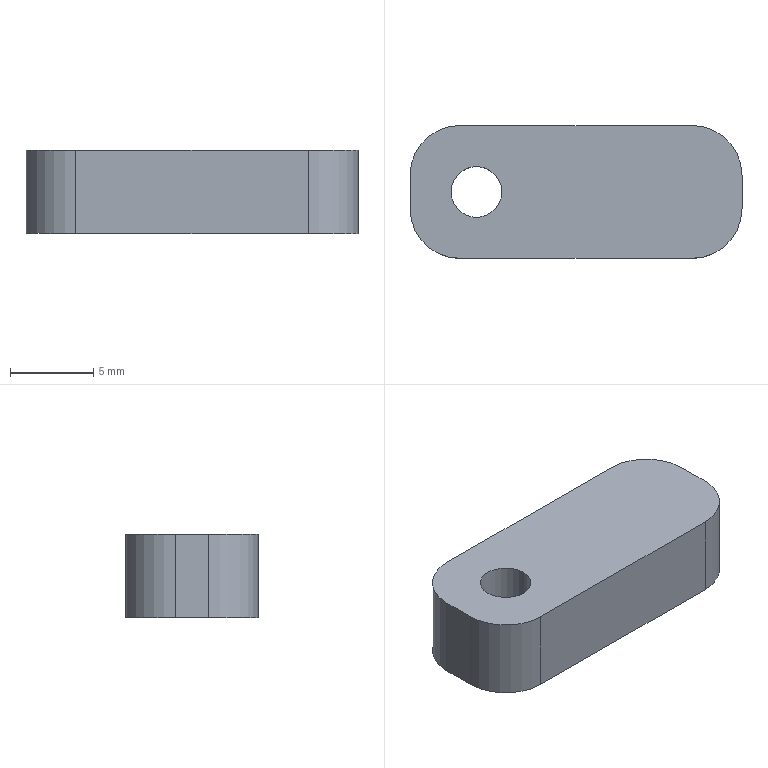Part | STEP file | ASND-0110-7.2aq | 1 solid | 12 faces | box 20 x 8 x 5 mm | volume 724.735 mm3 | cylinder 6 | plane 6 | commonest cylinder face diameters 6 x4 3.054 x2
STEP:
#1=CARTESIAN_POINT('',(0.,0.,0.));
#2=DIRECTION('',(0.,0.,1.));
#3=DIRECTION('',(1.,0.,0.));
#4=AXIS2_PLACEMENT_3D('',#1,#2,#3);
#5=CARTESIAN_POINT('',(-7.527,0.,5.));
#6=VERTEX_POINT('',#5);
#7=CARTESIAN_POINT('',(-7.527,0.,0.));
#8=VERTEX_POINT('',#7);
#9=CARTESIAN_POINT('',(-7.527,0.,5.));
#10=DIRECTION('',(0.,0.,-1.));
#11=VECTOR('',#10,1.);
#12=LINE('',#9,#11);
#13=CARTESIAN_POINT('',(-6.,0.,5.));
#14=DIRECTION('',(0.,0.,-1.));
#15=DIRECTION('',(-1.,0.,0.));
#16=AXIS2_PLACEMENT_3D('',#13,#14,#15);
#17=CYLINDRICAL_SURFACE('',#16,1.527);
#18=CARTESIAN_POINT('',(6.283,0.));
#19=DIRECTION('',(0.,1.));
#20=VECTOR('',#19,1.);
#21=LINE('',#18,#20);
#22=(GEOMETRIC_REPRESENTATION_CONTEXT(2)PARAMETRIC_REPRESENTATION_CONTEXT()REPRESENTATION_CONTEXT('',''));
#23=DEFINITIONAL_REPRESENTATION('',(#21),#22);
#24=PCURVE('',#17,#23);
#25=CARTESIAN_POINT('',(-6.,0.,5.));
#26=DIRECTION('',(0.,0.,-1.));
#27=DIRECTION('',(-1.,0.,0.));
#28=AXIS2_PLACEMENT_3D('',#25,#26,#27);
#29=CYLINDRICAL_SURFACE('',#28,1.527);
#30=CARTESIAN_POINT('',(0.,0.));
#31=DIRECTION('',(0.,1.));
#32=VECTOR('',#31,1.);
#33=LINE('',#30,#32);
#34=(GEOMETRIC_REPRESENTATION_CONTEXT(2)PARAMETRIC_REPRESENTATION_CONTEXT()REPRESENTATION_CONTEXT('',''));
#35=DEFINITIONAL_REPRESENTATION('',(#33),#34);
#36=PCURVE('',#29,#35);
#37=SURFACE_CURVE('',#12,(#24,#36),.PCURVE_S1.);
#38=EDGE_CURVE('',#6,#8,#37,.T.);
#39=ORIENTED_EDGE('',*,*,#38,.T.);
#40=CARTESIAN_POINT('',(-4.473,0.,0.));
#41=VERTEX_POINT('',#40);
#42=CARTESIAN_POINT('',(-6.,0.,0.));
#43=DIRECTION('',(0.,0.,1.));
#44=DIRECTION('',(1.,0.,0.));
#45=AXIS2_PLACEMENT_3D('',#42,#43,#44);
#46=CIRCLE('',#45,1.527);
#47=CARTESIAN_POINT('',(9.425,5.));
#48=DIRECTION('',(-1.,0.));
#49=VECTOR('',#48,1.);
#50=LINE('',#47,#49);
#51=(GEOMETRIC_REPRESENTATION_CONTEXT(2)PARAMETRIC_REPRESENTATION_CONTEXT()REPRESENTATION_CONTEXT('',''));
#52=DEFINITIONAL_REPRESENTATION('',(#50),#51);
#53=PCURVE('',#17,#52);
#54=CARTESIAN_POINT('',(0.,0.,0.));
#55=DIRECTION('',(0.,0.,-1.));
#56=DIRECTION('',(0.7071,0.7071,0.));
#57=AXIS2_PLACEMENT_3D('',#54,#55,#56);
#58=PLANE('',#57);
#59=CARTESIAN_POINT('',(-3.163,-3.163));
#60=CARTESIAN_POINT('',(-1.292,-5.033));
#61=CARTESIAN_POINT('',(-3.847,-5.718));
#62=CARTESIAN_POINT('',(-6.402,-6.402));
#63=CARTESIAN_POINT('',(-5.718,-3.847));
#64=CARTESIAN_POINT('',(-5.033,-1.292));
#65=CARTESIAN_POINT('',(-3.163,-3.163));
#66=(BOUNDED_CURVE()B_SPLINE_CURVE(2,(#59,#60,#61,#62,#63,#64,#65),.UNSPECIFIED.,.T.,.F.)B_SPLINE_CURVE_WITH_KNOTS((1,2,2,2,2,1),(-2.094,0.,2.094,4.189,6.283,8.378),.UNSPECIFIED.)CURVE()GEOMETRIC_REPRESENTATION_ITEM()RATIONAL_B_SPLINE_CURVE((1.,0.5,1.,0.5,1.,0.5,1.))REPRESENTATION_ITEM(''));
#67=(GEOMETRIC_REPRESENTATION_CONTEXT(2)PARAMETRIC_REPRESENTATION_CONTEXT()REPRESENTATION_CONTEXT('',''));
#68=DEFINITIONAL_REPRESENTATION('',(#66),#67);
#69=PCURVE('',#58,#68);
#70=SURFACE_CURVE('',#46,(#53,#69),.PCURVE_S1.);
#71=EDGE_CURVE('',#8,#41,#70,.T.);
#72=ORIENTED_EDGE('',*,*,#71,.T.);
#73=CARTESIAN_POINT('',(-4.473,0.,5.));
#74=VERTEX_POINT('',#73);
#75=CARTESIAN_POINT('',(-4.473,0.,5.));
#76=DIRECTION('',(0.,0.,-1.));
#77=VECTOR('',#76,1.);
#78=LINE('',#75,#77);
#79=CARTESIAN_POINT('',(3.142,0.));
#80=DIRECTION('',(0.,1.));
#81=VECTOR('',#80,1.);
#82=LINE('',#79,#81);
#83=(GEOMETRIC_REPRESENTATION_CONTEXT(2)PARAMETRIC_REPRESENTATION_CONTEXT()REPRESENTATION_CONTEXT('',''));
#84=DEFINITIONAL_REPRESENTATION('',(#82),#83);
#85=PCURVE('',#17,#84);
#86=CARTESIAN_POINT('',(3.142,0.));
#87=DIRECTION('',(0.,1.));
#88=VECTOR('',#87,1.);
#89=LINE('',#86,#88);
#90=(GEOMETRIC_REPRESENTATION_CONTEXT(2)PARAMETRIC_REPRESENTATION_CONTEXT()REPRESENTATION_CONTEXT('',''));
#91=DEFINITIONAL_REPRESENTATION('',(#89),#90);
#92=PCURVE('',#29,#91);
#93=SURFACE_CURVE('',#78,(#85,#92),.PCURVE_S1.);
#94=EDGE_CURVE('',#74,#41,#93,.T.);
#95=ORIENTED_EDGE('',*,*,#94,.F.);
#96=CARTESIAN_POINT('',(-6.,0.,5.));
#97=DIRECTION('',(0.,0.,1.));
#98=DIRECTION('',(1.,0.,0.));
#99=AXIS2_PLACEMENT_3D('',#96,#97,#98);
#100=CIRCLE('',#99,1.527);
#101=CARTESIAN_POINT('',(9.425,0.));
#102=DIRECTION('',(-1.,0.));
#103=VECTOR('',#102,1.);
#104=LINE('',#101,#103);
#105=(GEOMETRIC_REPRESENTATION_CONTEXT(2)PARAMETRIC_REPRESENTATION_CONTEXT()REPRESENTATION_CONTEXT('',''));
#106=DEFINITIONAL_REPRESENTATION('',(#104),#105);
#107=PCURVE('',#17,#106);
#108=CARTESIAN_POINT('',(0.,0.,5.));
#109=DIRECTION('',(0.,0.,-1.));
#110=DIRECTION('',(0.7071,0.7071,0.));
#111=AXIS2_PLACEMENT_3D('',#108,#109,#110);
#112=PLANE('',#111);
#113=CARTESIAN_POINT('',(-3.163,-3.163));
#114=CARTESIAN_POINT('',(-1.292,-5.033));
#115=CARTESIAN_POINT('',(-3.847,-5.718));
#116=CARTESIAN_POINT('',(-6.402,-6.402));
#117=CARTESIAN_POINT('',(-5.718,-3.847));
#118=CARTESIAN_POINT('',(-5.033,-1.292));
#119=CARTESIAN_POINT('',(-3.163,-3.163));
#120=(BOUNDED_CURVE()B_SPLINE_CURVE(2,(#113,#114,#115,#116,#117,#118,#119),.UNSPECIFIED.,.T.,.F.)B_SPLINE_CURVE_WITH_KNOTS((1,2,2,2,2,1),(-2.094,0.,2.094,4.189,6.283,8.378),.UNSPECIFIED.)CURVE()GEOMETRIC_REPRESENTATION_ITEM()RATIONAL_B_SPLINE_CURVE((1.,0.5,1.,0.5,1.,0.5,1.))REPRESENTATION_ITEM(''));
#121=(GEOMETRIC_REPRESENTATION_CONTEXT(2)PARAMETRIC_REPRESENTATION_CONTEXT()REPRESENTATION_CONTEXT('',''));
#122=DEFINITIONAL_REPRESENTATION('',(#120),#121);
#123=PCURVE('',#112,#122);
#124=SURFACE_CURVE('',#100,(#107,#123),.PCURVE_S1.);
#125=EDGE_CURVE('',#6,#74,#124,.T.);
#126=ORIENTED_EDGE('',*,*,#125,.F.);
#127=EDGE_LOOP('',(#39,#72,#95,#126));
#128=FACE_BOUND('',#127,.F.);
#129=ADVANCED_FACE('',(#128),#17,.F.);
#130=CARTESIAN_POINT('',(10.,-1.,5.));
#131=VERTEX_POINT('',#130);
#132=CARTESIAN_POINT('',(10.,1.,5.));
#133=VERTEX_POINT('',#132);
#134=CARTESIAN_POINT('',(10.,-1.,5.));
#135=DIRECTION('',(0.,1.,0.));
#136=VECTOR('',#135,1.);
#137=LINE('',#134,#136);
#138=CARTESIAN_POINT('',(6.364,7.778));
#139=DIRECTION('',(0.7071,-0.7071));
#140=VECTOR('',#139,1.);
#141=LINE('',#138,#140);
#142=(GEOMETRIC_REPRESENTATION_CONTEXT(2)PARAMETRIC_REPRESENTATION_CONTEXT()REPRESENTATION_CONTEXT('',''));
#143=DEFINITIONAL_REPRESENTATION('',(#141),#142);
#144=PCURVE('',#112,#143);
#145=CARTESIAN_POINT('',(10.,-4.,5.));
#146=DIRECTION('',(-1.,0.,0.));
#147=DIRECTION('',(0.,0.7071,0.7071));
#148=AXIS2_PLACEMENT_3D('',#145,#146,#147);
#149=PLANE('',#148);
#150=CARTESIAN_POINT('',(2.121,2.121));
#151=DIRECTION('',(0.7071,0.7071));
#152=VECTOR('',#151,1.);
#153=LINE('',#150,#152);
#154=(GEOMETRIC_REPRESENTATION_CONTEXT(2)PARAMETRIC_REPRESENTATION_CONTEXT()REPRESENTATION_CONTEXT('',''));
#155=DEFINITIONAL_REPRESENTATION('',(#153),#154);
#156=PCURVE('',#149,#155);
#157=SURFACE_CURVE('',#137,(#144,#156),.PCURVE_S1.);
#158=EDGE_CURVE('',#131,#133,#157,.T.);
#159=ORIENTED_EDGE('',*,*,#158,.T.);
#160=CARTESIAN_POINT('',(7.,4.,5.));
#161=VERTEX_POINT('',#160);
#162=CARTESIAN_POINT('',(7.,1.,5.));
#163=DIRECTION('',(0.,0.,1.));
#164=DIRECTION('',(-1.,0.,0.));
#165=AXIS2_PLACEMENT_3D('',#162,#163,#164);
#166=CIRCLE('',#165,3.);
#167=CARTESIAN_POINT('',(3.536,2.121));
#168=CARTESIAN_POINT('',(-0.1387,5.796));
#169=CARTESIAN_POINT('',(4.88,7.14));
#170=CARTESIAN_POINT('',(9.899,8.485));
#171=CARTESIAN_POINT('',(8.555,3.466));
#172=CARTESIAN_POINT('',(7.21,-1.553));
#173=CARTESIAN_POINT('',(3.536,2.121));
#174=(BOUNDED_CURVE()B_SPLINE_CURVE(2,(#167,#168,#169,#170,#171,#172,#173),.UNSPECIFIED.,.T.,.F.)B_SPLINE_CURVE_WITH_KNOTS((1,2,2,2,2,1),(-2.094,0.,2.094,4.189,6.283,8.378),.UNSPECIFIED.)CURVE()GEOMETRIC_REPRESENTATION_ITEM()RATIONAL_B_SPLINE_CURVE((1.,0.5,1.,0.5,1.,0.5,1.))REPRESENTATION_ITEM(''));
#175=(GEOMETRIC_REPRESENTATION_CONTEXT(2)PARAMETRIC_REPRESENTATION_CONTEXT()REPRESENTATION_CONTEXT('',''));
#176=DEFINITIONAL_REPRESENTATION('',(#174),#175);
#177=PCURVE('',#112,#176);
#178=CARTESIAN_POINT('',(7.,1.,5.));
#179=DIRECTION('',(0.,0.,-1.));
#180=DIRECTION('',(-1.,0.,0.));
#181=AXIS2_PLACEMENT_3D('',#178,#179,#180);
#182=CYLINDRICAL_SURFACE('',#181,3.);
#183=CARTESIAN_POINT('',(6.283,0.));
#184=DIRECTION('',(-1.,0.));
#185=VECTOR('',#184,1.);
#186=LINE('',#183,#185);
#187=(GEOMETRIC_REPRESENTATION_CONTEXT(2)PARAMETRIC_REPRESENTATION_CONTEXT()REPRESENTATION_CONTEXT('',''));
#188=DEFINITIONAL_REPRESENTATION('',(#186),#187);
#189=PCURVE('',#182,#188);
#190=SURFACE_CURVE('',#166,(#177,#189),.PCURVE_S1.);
#191=EDGE_CURVE('',#133,#161,#190,.T.);
#192=ORIENTED_EDGE('',*,*,#191,.T.);
#193=CARTESIAN_POINT('',(-7.,4.,5.));
#194=VERTEX_POINT('',#193);
#195=CARTESIAN_POINT('',(7.,4.,5.));
#196=DIRECTION('',(-1.,0.,0.));
#197=VECTOR('',#196,1.);
#198=LINE('',#195,#197);
#199=CARTESIAN_POINT('',(7.778,2.121));
#200=DIRECTION('',(-0.7071,-0.7071));
#201=VECTOR('',#200,1.);
#202=LINE('',#199,#201);
#203=(GEOMETRIC_REPRESENTATION_CONTEXT(2)PARAMETRIC_REPRESENTATION_CONTEXT()REPRESENTATION_CONTEXT('',''));
#204=DEFINITIONAL_REPRESENTATION('',(#202),#203);
#205=PCURVE('',#112,#204);
#206=CARTESIAN_POINT('',(-10.,4.,5.));
#207=DIRECTION('',(0.,-1.,0.));
#208=DIRECTION('',(0.7071,0.,0.7071));
#209=AXIS2_PLACEMENT_3D('',#206,#207,#208);
#210=PLANE('',#209);
#211=CARTESIAN_POINT('',(12.021,-12.021));
#212=DIRECTION('',(-0.7071,0.7071));
#213=VECTOR('',#212,1.);
#214=LINE('',#211,#213);
#215=(GEOMETRIC_REPRESENTATION_CONTEXT(2)PARAMETRIC_REPRESENTATION_CONTEXT()REPRESENTATION_CONTEXT('',''));
#216=DEFINITIONAL_REPRESENTATION('',(#214),#215);
#217=PCURVE('',#210,#216);
#218=SURFACE_CURVE('',#198,(#205,#217),.PCURVE_S1.);
#219=EDGE_CURVE('',#161,#194,#218,.T.);
#220=ORIENTED_EDGE('',*,*,#219,.T.);
#221=CARTESIAN_POINT('',(-10.,1.,5.));
#222=VERTEX_POINT('',#221);
#223=CARTESIAN_POINT('',(-7.,1.,5.));
#224=DIRECTION('',(0.,0.,1.));
#225=DIRECTION('',(-1.,0.,0.));
#226=AXIS2_PLACEMENT_3D('',#223,#224,#225);
#227=CIRCLE('',#226,3.);
#228=CARTESIAN_POINT('',(-6.364,-7.778));
#229=CARTESIAN_POINT('',(-10.038,-4.104));
#230=CARTESIAN_POINT('',(-5.019,-2.759));
#231=CARTESIAN_POINT('',(0.,-1.414));
#232=CARTESIAN_POINT('',(-1.345,-6.433));
#233=CARTESIAN_POINT('',(-2.69,-11.452));
#234=CARTESIAN_POINT('',(-6.364,-7.778));
#235=(BOUNDED_CURVE()B_SPLINE_CURVE(2,(#228,#229,#230,#231,#232,#233,#234),.UNSPECIFIED.,.T.,.F.)B_SPLINE_CURVE_WITH_KNOTS((1,2,2,2,2,1),(-2.094,0.,2.094,4.189,6.283,8.378),.UNSPECIFIED.)CURVE()GEOMETRIC_REPRESENTATION_ITEM()RATIONAL_B_SPLINE_CURVE((1.,0.5,1.,0.5,1.,0.5,1.))REPRESENTATION_ITEM(''));
#236=(GEOMETRIC_REPRESENTATION_CONTEXT(2)PARAMETRIC_REPRESENTATION_CONTEXT()REPRESENTATION_CONTEXT('',''));
#237=DEFINITIONAL_REPRESENTATION('',(#235),#236);
#238=PCURVE('',#112,#237);
#239=CARTESIAN_POINT('',(-7.,1.,5.));
#240=DIRECTION('',(0.,0.,-1.));
#241=DIRECTION('',(-1.,0.,0.));
#242=AXIS2_PLACEMENT_3D('',#239,#240,#241);
#243=CYLINDRICAL_SURFACE('',#242,3.);
#244=CARTESIAN_POINT('',(6.283,0.));
#245=DIRECTION('',(-1.,0.));
#246=VECTOR('',#245,1.);
#247=LINE('',#244,#246);
#248=(GEOMETRIC_REPRESENTATION_CONTEXT(2)PARAMETRIC_REPRESENTATION_CONTEXT()REPRESENTATION_CONTEXT('',''));
#249=DEFINITIONAL_REPRESENTATION('',(#247),#248);
#250=PCURVE('',#243,#249);
#251=SURFACE_CURVE('',#227,(#238,#250),.PCURVE_S1.);
#252=EDGE_CURVE('',#194,#222,#251,.T.);
#253=ORIENTED_EDGE('',*,*,#252,.T.);
#254=CARTESIAN_POINT('',(-10.,-1.,5.));
#255=VERTEX_POINT('',#254);
#256=CARTESIAN_POINT('',(-10.,1.,5.));
#257=DIRECTION('',(0.,-1.,0.));
#258=VECTOR('',#257,1.);
#259=LINE('',#256,#258);
#260=CARTESIAN_POINT('',(-6.364,-7.778));
#261=DIRECTION('',(-0.7071,0.7071));
#262=VECTOR('',#261,1.);
#263=LINE('',#260,#262);
#264=(GEOMETRIC_REPRESENTATION_CONTEXT(2)PARAMETRIC_REPRESENTATION_CONTEXT()REPRESENTATION_CONTEXT('',''));
#265=DEFINITIONAL_REPRESENTATION('',(#263),#264);
#266=PCURVE('',#112,#265);
#267=CARTESIAN_POINT('',(-10.,-4.,5.));
#268=DIRECTION('',(1.,0.,0.));
#269=DIRECTION('',(0.,0.7071,0.7071));
#270=AXIS2_PLACEMENT_3D('',#267,#268,#269);
#271=PLANE('',#270);
#272=CARTESIAN_POINT('',(3.536,-3.536));
#273=DIRECTION('',(-0.7071,0.7071));
#274=VECTOR('',#273,1.);
#275=LINE('',#272,#274);
#276=(GEOMETRIC_REPRESENTATION_CONTEXT(2)PARAMETRIC_REPRESENTATION_CONTEXT()REPRESENTATION_CONTEXT('',''));
#277=DEFINITIONAL_REPRESENTATION('',(#275),#276);
#278=PCURVE('',#271,#277);
#279=SURFACE_CURVE('',#259,(#266,#278),.PCURVE_S1.);
#280=EDGE_CURVE('',#222,#255,#279,.T.);
#281=ORIENTED_EDGE('',*,*,#280,.T.);
#282=CARTESIAN_POINT('',(-7.,-4.,5.));
#283=VERTEX_POINT('',#282);
#284=CARTESIAN_POINT('',(-7.,-1.,5.));
#285=DIRECTION('',(0.,0.,1.));
#286=DIRECTION('',(-1.,0.,0.));
#287=AXIS2_PLACEMENT_3D('',#284,#285,#286);
#288=CIRCLE('',#287,3.);
#289=CARTESIAN_POINT('',(-7.778,-6.364));
#290=CARTESIAN_POINT('',(-11.452,-2.69));
#291=CARTESIAN_POINT('',(-6.433,-1.345));
#292=CARTESIAN_POINT('',(-1.414,0.));
#293=CARTESIAN_POINT('',(-2.759,-5.019));
#294=CARTESIAN_POINT('',(-4.104,-10.038));
#295=CARTESIAN_POINT('',(-7.778,-6.364));
#296=(BOUNDED_CURVE()B_SPLINE_CURVE(2,(#289,#290,#291,#292,#293,#294,#295),.UNSPECIFIED.,.T.,.F.)B_SPLINE_CURVE_WITH_KNOTS((1,2,2,2,2,1),(-2.094,0.,2.094,4.189,6.283,8.378),.UNSPECIFIED.)CURVE()GEOMETRIC_REPRESENTATION_ITEM()RATIONAL_B_SPLINE_CURVE((1.,0.5,1.,0.5,1.,0.5,1.))REPRESENTATION_ITEM(''));
#297=(GEOMETRIC_REPRESENTATION_CONTEXT(2)PARAMETRIC_REPRESENTATION_CONTEXT()REPRESENTATION_CONTEXT('',''));
#298=DEFINITIONAL_REPRESENTATION('',(#296),#297);
#299=PCURVE('',#112,#298);
#300=CARTESIAN_POINT('',(-7.,-1.,5.));
#301=DIRECTION('',(0.,0.,-1.));
#302=DIRECTION('',(-1.,0.,0.));
#303=AXIS2_PLACEMENT_3D('',#300,#301,#302);
#304=CYLINDRICAL_SURFACE('',#303,3.);
#305=CARTESIAN_POINT('',(6.283,0.));
#306=DIRECTION('',(-1.,0.));
#307=VECTOR('',#306,1.);
#308=LINE('',#305,#307);
#309=(GEOMETRIC_REPRESENTATION_CONTEXT(2)PARAMETRIC_REPRESENTATION_CONTEXT()REPRESENTATION_CONTEXT('',''));
#310=DEFINITIONAL_REPRESENTATION('',(#308),#309);
#311=PCURVE('',#304,#310);
#312=SURFACE_CURVE('',#288,(#299,#311),.PCURVE_S1.);
#313=EDGE_CURVE('',#255,#283,#312,.T.);
#314=ORIENTED_EDGE('',*,*,#313,.T.);
#315=CARTESIAN_POINT('',(7.,-4.,5.));
#316=VERTEX_POINT('',#315);
#317=CARTESIAN_POINT('',(-7.,-4.,5.));
#318=DIRECTION('',(1.,0.,0.));
#319=VECTOR('',#318,1.);
#320=LINE('',#317,#319);
#321=CARTESIAN_POINT('',(-7.778,-2.121));
#322=DIRECTION('',(0.7071,0.7071));
#323=VECTOR('',#322,1.);
#324=LINE('',#321,#323);
#325=(GEOMETRIC_REPRESENTATION_CONTEXT(2)PARAMETRIC_REPRESENTATION_CONTEXT()REPRESENTATION_CONTEXT('',''));
#326=DEFINITIONAL_REPRESENTATION('',(#324),#325);
#327=PCURVE('',#112,#326);
#328=CARTESIAN_POINT('',(-10.,-4.,5.));
#329=DIRECTION('',(0.,1.,0.));
#330=DIRECTION('',(0.7071,0.,0.7071));
#331=AXIS2_PLACEMENT_3D('',#328,#329,#330);
#332=PLANE('',#331);
#333=CARTESIAN_POINT('',(2.121,2.121));
#334=DIRECTION('',(0.7071,0.7071));
#335=VECTOR('',#334,1.);
#336=LINE('',#333,#335);
#337=(GEOMETRIC_REPRESENTATION_CONTEXT(2)PARAMETRIC_REPRESENTATION_CONTEXT()REPRESENTATION_CONTEXT('',''));
#338=DEFINITIONAL_REPRESENTATION('',(#336),#337);
#339=PCURVE('',#332,#338);
#340=SURFACE_CURVE('',#320,(#327,#339),.PCURVE_S1.);
#341=EDGE_CURVE('',#283,#316,#340,.T.);
#342=ORIENTED_EDGE('',*,*,#341,.T.);
#343=CARTESIAN_POINT('',(7.,-1.,5.));
#344=DIRECTION('',(0.,0.,1.));
#345=DIRECTION('',(-1.,0.,0.));
#346=AXIS2_PLACEMENT_3D('',#343,#344,#345);
#347=CIRCLE('',#346,3.);
#348=CARTESIAN_POINT('',(2.121,3.536));
#349=CARTESIAN_POINT('',(-1.553,7.21));
#350=CARTESIAN_POINT('',(3.466,8.555));
#351=CARTESIAN_POINT('',(8.485,9.899));
#352=CARTESIAN_POINT('',(7.14,4.88));
#353=CARTESIAN_POINT('',(5.796,-0.1387));
#354=CARTESIAN_POINT('',(2.121,3.536));
#355=(BOUNDED_CURVE()B_SPLINE_CURVE(2,(#348,#349,#350,#351,#352,#353,#354),.UNSPECIFIED.,.T.,.F.)B_SPLINE_CURVE_WITH_KNOTS((1,2,2,2,2,1),(-2.094,0.,2.094,4.189,6.283,8.378),.UNSPECIFIED.)CURVE()GEOMETRIC_REPRESENTATION_ITEM()RATIONAL_B_SPLINE_CURVE((1.,0.5,1.,0.5,1.,0.5,1.))REPRESENTATION_ITEM(''));
#356=(GEOMETRIC_REPRESENTATION_CONTEXT(2)PARAMETRIC_REPRESENTATION_CONTEXT()REPRESENTATION_CONTEXT('',''));
#357=DEFINITIONAL_REPRESENTATION('',(#355),#356);
#358=PCURVE('',#112,#357);
#359=CARTESIAN_POINT('',(7.,-1.,5.));
#360=DIRECTION('',(0.,0.,-1.));
#361=DIRECTION('',(-1.,0.,0.));
#362=AXIS2_PLACEMENT_3D('',#359,#360,#361);
#363=CYLINDRICAL_SURFACE('',#362,3.);
#364=CARTESIAN_POINT('',(6.283,0.));
#365=DIRECTION('',(-1.,0.));
#366=VECTOR('',#365,1.);
#367=LINE('',#364,#366);
#368=(GEOMETRIC_REPRESENTATION_CONTEXT(2)PARAMETRIC_REPRESENTATION_CONTEXT()REPRESENTATION_CONTEXT('',''));
#369=DEFINITIONAL_REPRESENTATION('',(#367),#368);
#370=PCURVE('',#363,#369);
#371=SURFACE_CURVE('',#347,(#358,#370),.PCURVE_S1.);
#372=EDGE_CURVE('',#316,#131,#371,.T.);
#373=ORIENTED_EDGE('',*,*,#372,.T.);
#374=EDGE_LOOP('',(#159,#192,#220,#253,#281,#314,#342,#373));
#375=FACE_BOUND('',#374,.T.);
#376=ORIENTED_EDGE('',*,*,#125,.F.);
#377=CARTESIAN_POINT('',(-6.,0.,5.));
#378=DIRECTION('',(0.,0.,1.));
#379=DIRECTION('',(1.,0.,0.));
#380=AXIS2_PLACEMENT_3D('',#377,#378,#379);
#381=CIRCLE('',#380,1.527);
#382=CARTESIAN_POINT('',(-3.163,-3.163));
#383=CARTESIAN_POINT('',(-1.292,-5.033));
#384=CARTESIAN_POINT('',(-3.847,-5.718));
#385=CARTESIAN_POINT('',(-6.402,-6.402));
#386=CARTESIAN_POINT('',(-5.718,-3.847));
#387=CARTESIAN_POINT('',(-5.033,-1.292));
#388=CARTESIAN_POINT('',(-3.163,-3.163));
#389=(BOUNDED_CURVE()B_SPLINE_CURVE(2,(#382,#383,#384,#385,#386,#387,#388),.UNSPECIFIED.,.T.,.F.)B_SPLINE_CURVE_WITH_KNOTS((1,2,2,2,2,1),(-2.094,0.,2.094,4.189,6.283,8.378),.UNSPECIFIED.)CURVE()GEOMETRIC_REPRESENTATION_ITEM()RATIONAL_B_SPLINE_CURVE((1.,0.5,1.,0.5,1.,0.5,1.))REPRESENTATION_ITEM(''));
#390=(GEOMETRIC_REPRESENTATION_CONTEXT(2)PARAMETRIC_REPRESENTATION_CONTEXT()REPRESENTATION_CONTEXT('',''));
#391=DEFINITIONAL_REPRESENTATION('',(#389),#390);
#392=PCURVE('',#112,#391);
#393=CARTESIAN_POINT('',(3.142,0.));
#394=DIRECTION('',(-1.,0.));
#395=VECTOR('',#394,1.);
#396=LINE('',#393,#395);
#397=(GEOMETRIC_REPRESENTATION_CONTEXT(2)PARAMETRIC_REPRESENTATION_CONTEXT()REPRESENTATION_CONTEXT('',''));
#398=DEFINITIONAL_REPRESENTATION('',(#396),#397);
#399=PCURVE('',#29,#398);
#400=SURFACE_CURVE('',#381,(#392,#399),.PCURVE_S1.);
#401=EDGE_CURVE('',#74,#6,#400,.T.);
#402=ORIENTED_EDGE('',*,*,#401,.F.);
#403=EDGE_LOOP('',(#376,#402));
#404=FACE_BOUND('',#403,.T.);
#405=ADVANCED_FACE('',(#375,#404),#112,.F.);
#406=CARTESIAN_POINT('',(7.,4.,0.));
#407=VERTEX_POINT('',#406);
#408=CARTESIAN_POINT('',(-7.,4.,0.));
#409=VERTEX_POINT('',#408);
#410=CARTESIAN_POINT('',(7.,4.,0.));
#411=DIRECTION('',(-1.,0.,0.));
#412=VECTOR('',#411,1.);
#413=LINE('',#410,#412);
#414=CARTESIAN_POINT('',(7.778,2.121));
#415=DIRECTION('',(-0.7071,-0.7071));
#416=VECTOR('',#415,1.);
#417=LINE('',#414,#416);
#418=(GEOMETRIC_REPRESENTATION_CONTEXT(2)PARAMETRIC_REPRESENTATION_CONTEXT()REPRESENTATION_CONTEXT('',''));
#419=DEFINITIONAL_REPRESENTATION('',(#417),#418);
#420=PCURVE('',#58,#419);
#421=CARTESIAN_POINT('',(8.485,-15.556));
#422=DIRECTION('',(-0.7071,0.7071));
#423=VECTOR('',#422,1.);
#424=LINE('',#421,#423);
#425=(GEOMETRIC_REPRESENTATION_CONTEXT(2)PARAMETRIC_REPRESENTATION_CONTEXT()REPRESENTATION_CONTEXT('',''));
#426=DEFINITIONAL_REPRESENTATION('',(#424),#425);
#427=PCURVE('',#210,#426);
#428=SURFACE_CURVE('',#413,(#420,#427),.PCURVE_S1.);
#429=EDGE_CURVE('',#407,#409,#428,.T.);
#430=ORIENTED_EDGE('',*,*,#429,.F.);
#431=CARTESIAN_POINT('',(10.,1.,0.));
#432=VERTEX_POINT('',#431);
#433=CARTESIAN_POINT('',(7.,1.,0.));
#434=DIRECTION('',(0.,0.,-1.));
#435=DIRECTION('',(-1.,0.,0.));
#436=AXIS2_PLACEMENT_3D('',#433,#434,#435);
#437=CIRCLE('',#436,3.);
#438=CARTESIAN_POINT('',(5.657,4.243));
#439=DIRECTION('',(-0.7071,-0.7071));
#440=AXIS2_PLACEMENT_2D('',#438,#439);
#441=CIRCLE('',#440,3.);
#442=(GEOMETRIC_REPRESENTATION_CONTEXT(2)PARAMETRIC_REPRESENTATION_CONTEXT()REPRESENTATION_CONTEXT('',''));
#443=DEFINITIONAL_REPRESENTATION('',(#441),#442);
#444=PCURVE('',#58,#443);
#445=CARTESIAN_POINT('',(0.,5.));
#446=DIRECTION('',(1.,0.));
#447=VECTOR('',#446,1.);
#448=LINE('',#445,#447);
#449=(GEOMETRIC_REPRESENTATION_CONTEXT(2)PARAMETRIC_REPRESENTATION_CONTEXT()REPRESENTATION_CONTEXT('',''));
#450=DEFINITIONAL_REPRESENTATION('',(#448),#449);
#451=PCURVE('',#182,#450);
#452=SURFACE_CURVE('',#437,(#444,#451),.PCURVE_S1.);
#453=EDGE_CURVE('',#407,#432,#452,.T.);
#454=ORIENTED_EDGE('',*,*,#453,.T.);
#455=CARTESIAN_POINT('',(10.,-1.,0.));
#456=VERTEX_POINT('',#455);
#457=CARTESIAN_POINT('',(10.,-1.,0.));
#458=DIRECTION('',(0.,1.,0.));
#459=VECTOR('',#458,1.);
#460=LINE('',#457,#459);
#461=CARTESIAN_POINT('',(6.364,7.778));
#462=DIRECTION('',(0.7071,-0.7071));
#463=VECTOR('',#462,1.);
#464=LINE('',#461,#463);
#465=(GEOMETRIC_REPRESENTATION_CONTEXT(2)PARAMETRIC_REPRESENTATION_CONTEXT()REPRESENTATION_CONTEXT('',''));
#466=DEFINITIONAL_REPRESENTATION('',(#464),#465);
#467=PCURVE('',#58,#466);
#468=CARTESIAN_POINT('',(-1.414,5.657));
#469=DIRECTION('',(0.7071,0.7071));
#470=VECTOR('',#469,1.);
#471=LINE('',#468,#470);
#472=(GEOMETRIC_REPRESENTATION_CONTEXT(2)PARAMETRIC_REPRESENTATION_CONTEXT()REPRESENTATION_CONTEXT('',''));
#473=DEFINITIONAL_REPRESENTATION('',(#471),#472);
#474=PCURVE('',#149,#473);
#475=SURFACE_CURVE('',#460,(#467,#474),.PCURVE_S1.);
#476=EDGE_CURVE('',#456,#432,#475,.T.);
#477=ORIENTED_EDGE('',*,*,#476,.F.);
#478=CARTESIAN_POINT('',(7.,-4.,0.));
#479=VERTEX_POINT('',#478);
#480=CARTESIAN_POINT('',(7.,-1.,0.));
#481=DIRECTION('',(0.,0.,-1.));
#482=DIRECTION('',(-1.,0.,0.));
#483=AXIS2_PLACEMENT_3D('',#480,#481,#482);
#484=CIRCLE('',#483,3.);
#485=CARTESIAN_POINT('',(4.243,5.657));
#486=DIRECTION('',(-0.7071,-0.7071));
#487=AXIS2_PLACEMENT_2D('',#485,#486);
#488=CIRCLE('',#487,3.);
#489=(GEOMETRIC_REPRESENTATION_CONTEXT(2)PARAMETRIC_REPRESENTATION_CONTEXT()REPRESENTATION_CONTEXT('',''));
#490=DEFINITIONAL_REPRESENTATION('',(#488),#489);
#491=PCURVE('',#58,#490);
#492=CARTESIAN_POINT('',(0.,5.));
#493=DIRECTION('',(1.,0.));
#494=VECTOR('',#493,1.);
#495=LINE('',#492,#494);
#496=(GEOMETRIC_REPRESENTATION_CONTEXT(2)PARAMETRIC_REPRESENTATION_CONTEXT()REPRESENTATION_CONTEXT('',''));
#497=DEFINITIONAL_REPRESENTATION('',(#495),#496);
#498=PCURVE('',#363,#497);
#499=SURFACE_CURVE('',#484,(#491,#498),.PCURVE_S1.);
#500=EDGE_CURVE('',#456,#479,#499,.T.);
#501=ORIENTED_EDGE('',*,*,#500,.T.);
#502=CARTESIAN_POINT('',(-7.,-4.,0.));
#503=VERTEX_POINT('',#502);
#504=CARTESIAN_POINT('',(-7.,-4.,0.));
#505=DIRECTION('',(1.,0.,0.));
#506=VECTOR('',#505,1.);
#507=LINE('',#504,#506);
#508=CARTESIAN_POINT('',(-7.778,-2.121));
#509=DIRECTION('',(0.7071,0.7071));
#510=VECTOR('',#509,1.);
#511=LINE('',#508,#510);
#512=(GEOMETRIC_REPRESENTATION_CONTEXT(2)PARAMETRIC_REPRESENTATION_CONTEXT()REPRESENTATION_CONTEXT('',''));
#513=DEFINITIONAL_REPRESENTATION('',(#511),#512);
#514=PCURVE('',#58,#513);
#515=CARTESIAN_POINT('',(-1.414,5.657));
#516=DIRECTION('',(0.7071,0.7071));
#517=VECTOR('',#516,1.);
#518=LINE('',#515,#517);
#519=(GEOMETRIC_REPRESENTATION_CONTEXT(2)PARAMETRIC_REPRESENTATION_CONTEXT()REPRESENTATION_CONTEXT('',''));
#520=DEFINITIONAL_REPRESENTATION('',(#518),#519);
#521=PCURVE('',#332,#520);
#522=SURFACE_CURVE('',#507,(#514,#521),.PCURVE_S1.);
#523=EDGE_CURVE('',#503,#479,#522,.T.);
#524=ORIENTED_EDGE('',*,*,#523,.F.);
#525=CARTESIAN_POINT('',(-10.,-1.,0.));
#526=VERTEX_POINT('',#525);
#527=CARTESIAN_POINT('',(-7.,-1.,0.));
#528=DIRECTION('',(0.,0.,-1.));
#529=DIRECTION('',(-1.,0.,0.));
#530=AXIS2_PLACEMENT_3D('',#527,#528,#529);
#531=CIRCLE('',#530,3.);
#532=CARTESIAN_POINT('',(-5.657,-4.243));
#533=DIRECTION('',(-0.7071,-0.7071));
#534=AXIS2_PLACEMENT_2D('',#532,#533);
#535=CIRCLE('',#534,3.);
#536=(GEOMETRIC_REPRESENTATION_CONTEXT(2)PARAMETRIC_REPRESENTATION_CONTEXT()REPRESENTATION_CONTEXT('',''));
#537=DEFINITIONAL_REPRESENTATION('',(#535),#536);
#538=PCURVE('',#58,#537);
#539=CARTESIAN_POINT('',(0.,5.));
#540=DIRECTION('',(1.,0.));
#541=VECTOR('',#540,1.);
#542=LINE('',#539,#541);
#543=(GEOMETRIC_REPRESENTATION_CONTEXT(2)PARAMETRIC_REPRESENTATION_CONTEXT()REPRESENTATION_CONTEXT('',''));
#544=DEFINITIONAL_REPRESENTATION('',(#542),#543);
#545=PCURVE('',#304,#544);
#546=SURFACE_CURVE('',#531,(#538,#545),.PCURVE_S1.);
#547=EDGE_CURVE('',#503,#526,#546,.T.);
#548=ORIENTED_EDGE('',*,*,#547,.T.);
#549=CARTESIAN_POINT('',(-10.,1.,0.));
#550=VERTEX_POINT('',#549);
#551=CARTESIAN_POINT('',(-10.,1.,0.));
#552=DIRECTION('',(0.,-1.,0.));
#553=VECTOR('',#552,1.);
#554=LINE('',#551,#553);
#555=CARTESIAN_POINT('',(-6.364,-7.778));
#556=DIRECTION('',(-0.7071,0.7071));
#557=VECTOR('',#556,1.);
#558=LINE('',#555,#557);
#559=(GEOMETRIC_REPRESENTATION_CONTEXT(2)PARAMETRIC_REPRESENTATION_CONTEXT()REPRESENTATION_CONTEXT('',''));
#560=DEFINITIONAL_REPRESENTATION('',(#558),#559);
#561=PCURVE('',#58,#560);
#562=CARTESIAN_POINT('',(0.,-7.071));
#563=DIRECTION('',(-0.7071,0.7071));
#564=VECTOR('',#563,1.);
#565=LINE('',#562,#564);
#566=(GEOMETRIC_REPRESENTATION_CONTEXT(2)PARAMETRIC_REPRESENTATION_CONTEXT()REPRESENTATION_CONTEXT('',''));
#567=DEFINITIONAL_REPRESENTATION('',(#565),#566);
#568=PCURVE('',#271,#567);
#569=SURFACE_CURVE('',#554,(#561,#568),.PCURVE_S1.);
#570=EDGE_CURVE('',#550,#526,#569,.T.);
#571=ORIENTED_EDGE('',*,*,#570,.F.);
#572=CARTESIAN_POINT('',(-7.,1.,0.));
#573=DIRECTION('',(0.,0.,-1.));
#574=DIRECTION('',(-1.,0.,0.));
#575=AXIS2_PLACEMENT_3D('',#572,#573,#574);
#576=CIRCLE('',#575,3.);
#577=CARTESIAN_POINT('',(-4.243,-5.657));
#578=DIRECTION('',(-0.7071,-0.7071));
#579=AXIS2_PLACEMENT_2D('',#577,#578);
#580=CIRCLE('',#579,3.);
#581=(GEOMETRIC_REPRESENTATION_CONTEXT(2)PARAMETRIC_REPRESENTATION_CONTEXT()REPRESENTATION_CONTEXT('',''));
#582=DEFINITIONAL_REPRESENTATION('',(#580),#581);
#583=PCURVE('',#58,#582);
#584=CARTESIAN_POINT('',(0.,5.));
#585=DIRECTION('',(1.,0.));
#586=VECTOR('',#585,1.);
#587=LINE('',#584,#586);
#588=(GEOMETRIC_REPRESENTATION_CONTEXT(2)PARAMETRIC_REPRESENTATION_CONTEXT()REPRESENTATION_CONTEXT('',''));
#589=DEFINITIONAL_REPRESENTATION('',(#587),#588);
#590=PCURVE('',#243,#589);
#591=SURFACE_CURVE('',#576,(#583,#590),.PCURVE_S1.);
#592=EDGE_CURVE('',#550,#409,#591,.T.);
#593=ORIENTED_EDGE('',*,*,#592,.T.);
#594=EDGE_LOOP('',(#430,#454,#477,#501,#524,#548,#571,#593));
#595=FACE_BOUND('',#594,.T.);
#596=ORIENTED_EDGE('',*,*,#71,.T.);
#597=CARTESIAN_POINT('',(-6.,0.,0.));
#598=DIRECTION('',(0.,0.,1.));
#599=DIRECTION('',(1.,0.,0.));
#600=AXIS2_PLACEMENT_3D('',#597,#598,#599);
#601=CIRCLE('',#600,1.527);
#602=CARTESIAN_POINT('',(-3.163,-3.163));
#603=CARTESIAN_POINT('',(-1.292,-5.033));
#604=CARTESIAN_POINT('',(-3.847,-5.718));
#605=CARTESIAN_POINT('',(-6.402,-6.402));
#606=CARTESIAN_POINT('',(-5.718,-3.847));
#607=CARTESIAN_POINT('',(-5.033,-1.292));
#608=CARTESIAN_POINT('',(-3.163,-3.163));
#609=(BOUNDED_CURVE()B_SPLINE_CURVE(2,(#602,#603,#604,#605,#606,#607,#608),.UNSPECIFIED.,.T.,.F.)B_SPLINE_CURVE_WITH_KNOTS((1,2,2,2,2,1),(-2.094,0.,2.094,4.189,6.283,8.378),.UNSPECIFIED.)CURVE()GEOMETRIC_REPRESENTATION_ITEM()RATIONAL_B_SPLINE_CURVE((1.,0.5,1.,0.5,1.,0.5,1.))REPRESENTATION_ITEM(''));
#610=(GEOMETRIC_REPRESENTATION_CONTEXT(2)PARAMETRIC_REPRESENTATION_CONTEXT()REPRESENTATION_CONTEXT('',''));
#611=DEFINITIONAL_REPRESENTATION('',(#609),#610);
#612=PCURVE('',#58,#611);
#613=CARTESIAN_POINT('',(3.142,5.));
#614=DIRECTION('',(-1.,0.));
#615=VECTOR('',#614,1.);
#616=LINE('',#613,#615);
#617=(GEOMETRIC_REPRESENTATION_CONTEXT(2)PARAMETRIC_REPRESENTATION_CONTEXT()REPRESENTATION_CONTEXT('',''));
#618=DEFINITIONAL_REPRESENTATION('',(#616),#617);
#619=PCURVE('',#29,#618);
#620=SURFACE_CURVE('',#601,(#612,#619),.PCURVE_S1.);
#621=EDGE_CURVE('',#41,#8,#620,.T.);
#622=ORIENTED_EDGE('',*,*,#621,.T.);
#623=EDGE_LOOP('',(#596,#622));
#624=FACE_BOUND('',#623,.T.);
#625=ADVANCED_FACE('',(#595,#624),#58,.T.);
#626=ORIENTED_EDGE('',*,*,#476,.T.);
#627=CARTESIAN_POINT('',(10.,1.,5.));
#628=DIRECTION('',(0.,0.,1.));
#629=VECTOR('',#628,1.);
#630=LINE('',#627,#629);
#631=CARTESIAN_POINT('',(3.536,3.536));
#632=DIRECTION('',(0.7071,-0.7071));
#633=VECTOR('',#632,1.);
#634=LINE('',#631,#633);
#635=(GEOMETRIC_REPRESENTATION_CONTEXT(2)PARAMETRIC_REPRESENTATION_CONTEXT()REPRESENTATION_CONTEXT('',''));
#636=DEFINITIONAL_REPRESENTATION('',(#634),#635);
#637=PCURVE('',#149,#636);
#638=CARTESIAN_POINT('',(3.142,0.));
#639=DIRECTION('',(0.,-1.));
#640=VECTOR('',#639,1.);
#641=LINE('',#638,#640);
#642=(GEOMETRIC_REPRESENTATION_CONTEXT(2)PARAMETRIC_REPRESENTATION_CONTEXT()REPRESENTATION_CONTEXT('',''));
#643=DEFINITIONAL_REPRESENTATION('',(#641),#642);
#644=PCURVE('',#182,#643);
#645=SURFACE_CURVE('',#630,(#637,#644),.PCURVE_S1.);
#646=EDGE_CURVE('',#432,#133,#645,.T.);
#647=ORIENTED_EDGE('',*,*,#646,.T.);
#648=ORIENTED_EDGE('',*,*,#158,.F.);
#649=CARTESIAN_POINT('',(10.,-1.,5.));
#650=DIRECTION('',(0.,0.,-1.));
#651=VECTOR('',#650,1.);
#652=LINE('',#649,#651);
#653=CARTESIAN_POINT('',(2.121,2.121));
#654=DIRECTION('',(-0.7071,0.7071));
#655=VECTOR('',#654,1.);
#656=LINE('',#653,#655);
#657=(GEOMETRIC_REPRESENTATION_CONTEXT(2)PARAMETRIC_REPRESENTATION_CONTEXT()REPRESENTATION_CONTEXT('',''));
#658=DEFINITIONAL_REPRESENTATION('',(#656),#657);
#659=PCURVE('',#149,#658);
#660=CARTESIAN_POINT('',(3.142,0.));
#661=DIRECTION('',(0.,1.));
#662=VECTOR('',#661,1.);
#663=LINE('',#660,#662);
#664=(GEOMETRIC_REPRESENTATION_CONTEXT(2)PARAMETRIC_REPRESENTATION_CONTEXT()REPRESENTATION_CONTEXT('',''));
#665=DEFINITIONAL_REPRESENTATION('',(#663),#664);
#666=PCURVE('',#363,#665);
#667=SURFACE_CURVE('',#652,(#659,#666),.PCURVE_S1.);
#668=EDGE_CURVE('',#131,#456,#667,.T.);
#669=ORIENTED_EDGE('',*,*,#668,.T.);
#670=EDGE_LOOP('',(#626,#647,#648,#669));
#671=FACE_BOUND('',#670,.T.);
#672=ADVANCED_FACE('',(#671),#149,.F.);
#673=ORIENTED_EDGE('',*,*,#219,.F.);
#674=CARTESIAN_POINT('',(7.,4.,5.));
#675=DIRECTION('',(0.,0.,-1.));
#676=VECTOR('',#675,1.);
#677=LINE('',#674,#676);
#678=CARTESIAN_POINT('',(12.021,-12.021));
#679=DIRECTION('',(-0.7071,-0.7071));
#680=VECTOR('',#679,1.);
#681=LINE('',#678,#680);
#682=(GEOMETRIC_REPRESENTATION_CONTEXT(2)PARAMETRIC_REPRESENTATION_CONTEXT()REPRESENTATION_CONTEXT('',''));
#683=DEFINITIONAL_REPRESENTATION('',(#681),#682);
#684=PCURVE('',#210,#683);
#685=CARTESIAN_POINT('',(1.571,0.));
#686=DIRECTION('',(0.,1.));
#687=VECTOR('',#686,1.);
#688=LINE('',#685,#687);
#689=(GEOMETRIC_REPRESENTATION_CONTEXT(2)PARAMETRIC_REPRESENTATION_CONTEXT()REPRESENTATION_CONTEXT('',''));
#690=DEFINITIONAL_REPRESENTATION('',(#688),#689);
#691=PCURVE('',#182,#690);
#692=SURFACE_CURVE('',#677,(#684,#691),.PCURVE_S1.);
#693=EDGE_CURVE('',#161,#407,#692,.T.);
#694=ORIENTED_EDGE('',*,*,#693,.T.);
#695=ORIENTED_EDGE('',*,*,#429,.T.);
#696=CARTESIAN_POINT('',(-7.,4.,5.));
#697=DIRECTION('',(0.,0.,1.));
#698=VECTOR('',#697,1.);
#699=LINE('',#696,#698);
#700=CARTESIAN_POINT('',(2.121,-2.121));
#701=DIRECTION('',(0.7071,0.7071));
#702=VECTOR('',#701,1.);
#703=LINE('',#700,#702);
#704=(GEOMETRIC_REPRESENTATION_CONTEXT(2)PARAMETRIC_REPRESENTATION_CONTEXT()REPRESENTATION_CONTEXT('',''));
#705=DEFINITIONAL_REPRESENTATION('',(#703),#704);
#706=PCURVE('',#210,#705);
#707=CARTESIAN_POINT('',(1.571,0.));
#708=DIRECTION('',(0.,-1.));
#709=VECTOR('',#708,1.);
#710=LINE('',#707,#709);
#711=(GEOMETRIC_REPRESENTATION_CONTEXT(2)PARAMETRIC_REPRESENTATION_CONTEXT()REPRESENTATION_CONTEXT('',''));
#712=DEFINITIONAL_REPRESENTATION('',(#710),#711);
#713=PCURVE('',#243,#712);
#714=SURFACE_CURVE('',#699,(#706,#713),.PCURVE_S1.);
#715=EDGE_CURVE('',#409,#194,#714,.T.);
#716=ORIENTED_EDGE('',*,*,#715,.T.);
#717=EDGE_LOOP('',(#673,#694,#695,#716));
#718=FACE_BOUND('',#717,.T.);
#719=ADVANCED_FACE('',(#718),#210,.F.);
#720=ORIENTED_EDGE('',*,*,#280,.F.);
#721=CARTESIAN_POINT('',(-10.,1.,5.));
#722=DIRECTION('',(0.,0.,-1.));
#723=VECTOR('',#722,1.);
#724=LINE('',#721,#723);
#725=CARTESIAN_POINT('',(3.536,-3.536));
#726=DIRECTION('',(-0.7071,-0.7071));
#727=VECTOR('',#726,1.);
#728=LINE('',#725,#727);
#729=(GEOMETRIC_REPRESENTATION_CONTEXT(2)PARAMETRIC_REPRESENTATION_CONTEXT()REPRESENTATION_CONTEXT('',''));
#730=DEFINITIONAL_REPRESENTATION('',(#728),#729);
#731=PCURVE('',#271,#730);
#732=CARTESIAN_POINT('',(0.,0.));
#733=DIRECTION('',(0.,1.));
#734=VECTOR('',#733,1.);
#735=LINE('',#732,#734);
#736=(GEOMETRIC_REPRESENTATION_CONTEXT(2)PARAMETRIC_REPRESENTATION_CONTEXT()REPRESENTATION_CONTEXT('',''));
#737=DEFINITIONAL_REPRESENTATION('',(#735),#736);
#738=PCURVE('',#243,#737);
#739=SURFACE_CURVE('',#724,(#731,#738),.PCURVE_S1.);
#740=EDGE_CURVE('',#222,#550,#739,.T.);
#741=ORIENTED_EDGE('',*,*,#740,.T.);
#742=ORIENTED_EDGE('',*,*,#570,.T.);
#743=CARTESIAN_POINT('',(-10.,-1.,5.));
#744=DIRECTION('',(0.,0.,1.));
#745=VECTOR('',#744,1.);
#746=LINE('',#743,#745);
#747=CARTESIAN_POINT('',(2.121,-2.121));
#748=DIRECTION('',(0.7071,0.7071));
#749=VECTOR('',#748,1.);
#750=LINE('',#747,#749);
#751=(GEOMETRIC_REPRESENTATION_CONTEXT(2)PARAMETRIC_REPRESENTATION_CONTEXT()REPRESENTATION_CONTEXT('',''));
#752=DEFINITIONAL_REPRESENTATION('',(#750),#751);
#753=PCURVE('',#271,#752);
#754=CARTESIAN_POINT('',(6.283,0.));
#755=DIRECTION('',(0.,-1.));
#756=VECTOR('',#755,1.);
#757=LINE('',#754,#756);
#758=(GEOMETRIC_REPRESENTATION_CONTEXT(2)PARAMETRIC_REPRESENTATION_CONTEXT()REPRESENTATION_CONTEXT('',''));
#759=DEFINITIONAL_REPRESENTATION('',(#757),#758);
#760=PCURVE('',#304,#759);
#761=SURFACE_CURVE('',#746,(#753,#760),.PCURVE_S1.);
#762=EDGE_CURVE('',#526,#255,#761,.T.);
#763=ORIENTED_EDGE('',*,*,#762,.T.);
#764=EDGE_LOOP('',(#720,#741,#742,#763));
#765=FACE_BOUND('',#764,.T.);
#766=ADVANCED_FACE('',(#765),#271,.F.);
#767=ORIENTED_EDGE('',*,*,#523,.T.);
#768=CARTESIAN_POINT('',(7.,-4.,5.));
#769=DIRECTION('',(0.,0.,1.));
#770=VECTOR('',#769,1.);
#771=LINE('',#768,#770);
#772=CARTESIAN_POINT('',(12.021,12.021));
#773=DIRECTION('',(0.7071,-0.7071));
#774=VECTOR('',#773,1.);
#775=LINE('',#772,#774);
#776=(GEOMETRIC_REPRESENTATION_CONTEXT(2)PARAMETRIC_REPRESENTATION_CONTEXT()REPRESENTATION_CONTEXT('',''));
#777=DEFINITIONAL_REPRESENTATION('',(#775),#776);
#778=PCURVE('',#332,#777);
#779=CARTESIAN_POINT('',(4.712,0.));
#780=DIRECTION('',(0.,-1.));
#781=VECTOR('',#780,1.);
#782=LINE('',#779,#781);
#783=(GEOMETRIC_REPRESENTATION_CONTEXT(2)PARAMETRIC_REPRESENTATION_CONTEXT()REPRESENTATION_CONTEXT('',''));
#784=DEFINITIONAL_REPRESENTATION('',(#782),#783);
#785=PCURVE('',#363,#784);
#786=SURFACE_CURVE('',#771,(#778,#785),.PCURVE_S1.);
#787=EDGE_CURVE('',#479,#316,#786,.T.);
#788=ORIENTED_EDGE('',*,*,#787,.T.);
#789=ORIENTED_EDGE('',*,*,#341,.F.);
#790=CARTESIAN_POINT('',(-7.,-4.,5.));
#791=DIRECTION('',(0.,0.,-1.));
#792=VECTOR('',#791,1.);
#793=LINE('',#790,#792);
#794=CARTESIAN_POINT('',(2.121,2.121));
#795=DIRECTION('',(-0.7071,0.7071));
#796=VECTOR('',#795,1.);
#797=LINE('',#794,#796);
#798=(GEOMETRIC_REPRESENTATION_CONTEXT(2)PARAMETRIC_REPRESENTATION_CONTEXT()REPRESENTATION_CONTEXT('',''));
#799=DEFINITIONAL_REPRESENTATION('',(#797),#798);
#800=PCURVE('',#332,#799);
#801=CARTESIAN_POINT('',(4.712,0.));
#802=DIRECTION('',(0.,1.));
#803=VECTOR('',#802,1.);
#804=LINE('',#801,#803);
#805=(GEOMETRIC_REPRESENTATION_CONTEXT(2)PARAMETRIC_REPRESENTATION_CONTEXT()REPRESENTATION_CONTEXT('',''));
#806=DEFINITIONAL_REPRESENTATION('',(#804),#805);
#807=PCURVE('',#304,#806);
#808=SURFACE_CURVE('',#793,(#800,#807),.PCURVE_S1.);
#809=EDGE_CURVE('',#283,#503,#808,.T.);
#810=ORIENTED_EDGE('',*,*,#809,.T.);
#811=EDGE_LOOP('',(#767,#788,#789,#810));
#812=FACE_BOUND('',#811,.T.);
#813=ADVANCED_FACE('',(#812),#332,.F.);
#814=ORIENTED_EDGE('',*,*,#621,.T.);
#815=ORIENTED_EDGE('',*,*,#38,.F.);
#816=ORIENTED_EDGE('',*,*,#401,.F.);
#817=ORIENTED_EDGE('',*,*,#94,.T.);
#818=EDGE_LOOP('',(#814,#815,#816,#817));
#819=FACE_BOUND('',#818,.F.);
#820=ADVANCED_FACE('',(#819),#29,.F.);
#821=ORIENTED_EDGE('',*,*,#191,.F.);
#822=ORIENTED_EDGE('',*,*,#646,.F.);
#823=ORIENTED_EDGE('',*,*,#453,.F.);
#824=ORIENTED_EDGE('',*,*,#693,.F.);
#825=EDGE_LOOP('',(#821,#822,#823,#824));
#826=FACE_BOUND('',#825,.T.);
#827=ADVANCED_FACE('',(#826),#182,.T.);
#828=ORIENTED_EDGE('',*,*,#372,.F.);
#829=ORIENTED_EDGE('',*,*,#787,.F.);
#830=ORIENTED_EDGE('',*,*,#500,.F.);
#831=ORIENTED_EDGE('',*,*,#668,.F.);
#832=EDGE_LOOP('',(#828,#829,#830,#831));
#833=FACE_BOUND('',#832,.T.);
#834=ADVANCED_FACE('',(#833),#363,.T.);
#835=ORIENTED_EDGE('',*,*,#252,.F.);
#836=ORIENTED_EDGE('',*,*,#715,.F.);
#837=ORIENTED_EDGE('',*,*,#592,.F.);
#838=ORIENTED_EDGE('',*,*,#740,.F.);
#839=EDGE_LOOP('',(#835,#836,#837,#838));
#840=FACE_BOUND('',#839,.T.);
#841=ADVANCED_FACE('',(#840),#243,.T.);
#842=ORIENTED_EDGE('',*,*,#313,.F.);
#843=ORIENTED_EDGE('',*,*,#762,.F.);
#844=ORIENTED_EDGE('',*,*,#547,.F.);
#845=ORIENTED_EDGE('',*,*,#809,.F.);
#846=EDGE_LOOP('',(#842,#843,#844,#845));
#847=FACE_BOUND('',#846,.T.);
#848=ADVANCED_FACE('',(#847),#304,.T.);
#849=CLOSED_SHELL('',(#129,#405,#625,#672,#719,#766,#813,#820,#827,#834,#841,#848));
#850=MANIFOLD_SOLID_BREP('',#849);
#851=(LENGTH_UNIT()NAMED_UNIT(*)SI_UNIT(.MILLI.,.METRE.));
#852=UNCERTAINTY_MEASURE_WITH_UNIT(LENGTH_MEASURE(0.0000001),#851,'','');
#853=(NAMED_UNIT(*)PLANE_ANGLE_UNIT()SI_UNIT($,.RADIAN.));
#854=(NAMED_UNIT(*)SI_UNIT($,.STERADIAN.)SOLID_ANGLE_UNIT());
#855=(GEOMETRIC_REPRESENTATION_CONTEXT(3)GLOBAL_UNCERTAINTY_ASSIGNED_CONTEXT((#852))GLOBAL_UNIT_ASSIGNED_CONTEXT((#851,#853,#854))REPRESENTATION_CONTEXT('',''));
#856=ADVANCED_BREP_SHAPE_REPRESENTATION('',(#4,#850),#855);